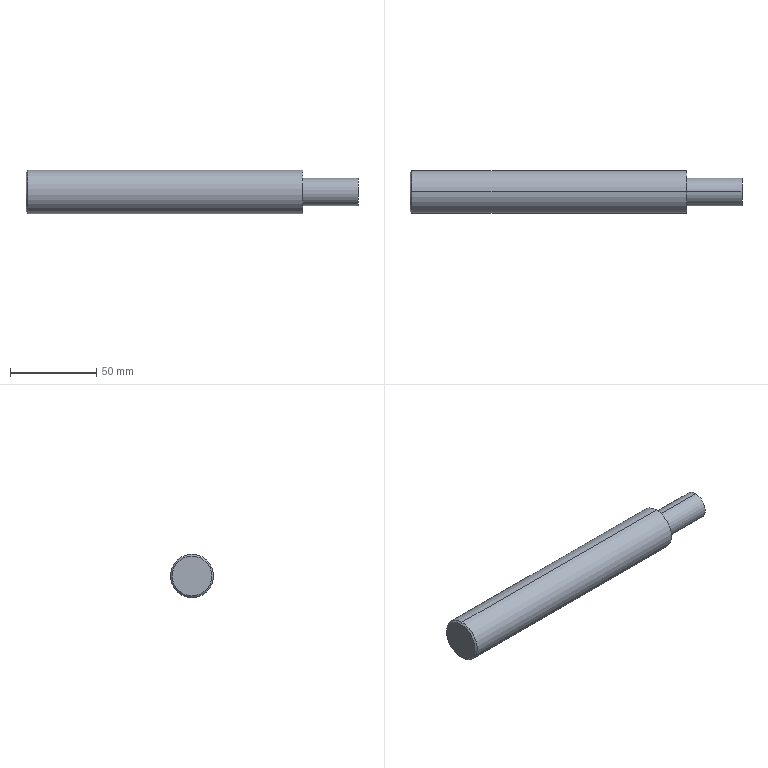Part | SolidWorks | features Chamfer 1, Revolution 1 | 1 solid | 9 faces | box 192 x 25 x 25 mm | volume 84936 mm3 | cylinder 4 | plane 3 | cone 2 | commonest cylinder face diameters 16 x2 25 x2
STEP:
#1=CARTESIAN_POINT('',(0.,0.,11.5));
#2=VERTEX_POINT('',#1);
#3=CARTESIAN_POINT('',(0.,0.,-11.5));
#4=VERTEX_POINT('',#3);
#5=CARTESIAN_POINT('',(0.,0.,0.));
#6=DIRECTION('',(-1.,0.,0.));
#7=DIRECTION('',(0.,0.,-1.));
#8=AXIS2_PLACEMENT_3D('',#5,#6,#7);
#9=CIRCLE('',#8,11.5);
#10=EDGE_CURVE('',#2,#4,#9,.T.);
#11=ORIENTED_EDGE('',*,*,#10,.F.);
#12=CARTESIAN_POINT('',(1.,0.,12.5));
#13=VERTEX_POINT('',#12);
#14=CARTESIAN_POINT('',(0.,0.,11.5));
#15=DIRECTION('',(0.7071,0.,0.7071));
#16=VECTOR('',#15,1000.);
#17=LINE('',#14,#16);
#18=EDGE_CURVE('',#2,#13,#17,.T.);
#19=ORIENTED_EDGE('',*,*,#18,.T.);
#20=CARTESIAN_POINT('',(1.,0.,-12.5));
#21=VERTEX_POINT('',#20);
#22=CARTESIAN_POINT('',(1.,0.,0.));
#23=DIRECTION('',(1.,0.,0.));
#24=DIRECTION('',(0.,0.,-1.));
#25=AXIS2_PLACEMENT_3D('',#22,#23,#24);
#26=CIRCLE('',#25,12.5);
#27=EDGE_CURVE('',#21,#13,#26,.T.);
#28=ORIENTED_EDGE('',*,*,#27,.F.);
#29=CARTESIAN_POINT('',(0.,0.,-11.5));
#30=DIRECTION('',(0.7071,0.,-0.7071));
#31=VECTOR('',#30,1000.);
#32=LINE('',#29,#31);
#33=EDGE_CURVE('',#4,#21,#32,.T.);
#34=ORIENTED_EDGE('',*,*,#33,.F.);
#35=EDGE_LOOP('',(#11,#19,#28,#34));
#36=FACE_OUTER_BOUND('',#35,.T.);
#37=CARTESIAN_POINT('',(0.,0.,0.));
#38=DIRECTION('',(1.,0.,0.));
#39=DIRECTION('',(0.,0.,-1.));
#40=AXIS2_PLACEMENT_3D('',#37,#38,#39);
#41=CONICAL_SURFACE('',#40,11.5,0.7854);
#42=ADVANCED_FACE('',(#36),#41,.T.);
#43=CARTESIAN_POINT('',(192.,0.,8.));
#44=VERTEX_POINT('',#43);
#45=CARTESIAN_POINT('',(192.,0.,-8.));
#46=VERTEX_POINT('',#45);
#47=CARTESIAN_POINT('',(192.,0.,0.));
#48=DIRECTION('',(-1.,0.,0.));
#49=DIRECTION('',(0.,0.,1.));
#50=AXIS2_PLACEMENT_3D('',#47,#48,#49);
#51=CIRCLE('',#50,8.);
#52=EDGE_CURVE('',#44,#46,#51,.T.);
#53=ORIENTED_EDGE('',*,*,#52,.T.);
#54=CARTESIAN_POINT('',(160.,0.,-8.));
#55=VERTEX_POINT('',#54);
#56=CARTESIAN_POINT('',(0.,0.,-8.));
#57=DIRECTION('',(-1.,0.,0.));
#58=VECTOR('',#57,1000.);
#59=LINE('',#56,#58);
#60=EDGE_CURVE('',#46,#55,#59,.T.);
#61=ORIENTED_EDGE('',*,*,#60,.T.);
#62=CARTESIAN_POINT('',(160.,0.,8.));
#63=VERTEX_POINT('',#62);
#64=CARTESIAN_POINT('',(160.,0.,0.));
#65=DIRECTION('',(-1.,0.,0.));
#66=DIRECTION('',(0.,0.,1.));
#67=AXIS2_PLACEMENT_3D('',#64,#65,#66);
#68=CIRCLE('',#67,8.);
#69=EDGE_CURVE('',#63,#55,#68,.T.);
#70=ORIENTED_EDGE('',*,*,#69,.F.);
#71=CARTESIAN_POINT('',(0.,0.,8.));
#72=DIRECTION('',(-1.,0.,0.));
#73=VECTOR('',#72,1000.);
#74=LINE('',#71,#73);
#75=EDGE_CURVE('',#44,#63,#74,.T.);
#76=ORIENTED_EDGE('',*,*,#75,.F.);
#77=EDGE_LOOP('',(#53,#61,#70,#76));
#78=FACE_OUTER_BOUND('',#77,.T.);
#79=CARTESIAN_POINT('',(0.,0.,0.));
#80=DIRECTION('',(-1.,0.,0.));
#81=DIRECTION('',(0.,0.,1.));
#82=AXIS2_PLACEMENT_3D('',#79,#80,#81);
#83=CYLINDRICAL_SURFACE('',#82,8.);
#84=ADVANCED_FACE('',(#78),#83,.T.);
#85=CARTESIAN_POINT('',(160.,0.,12.5));
#86=VERTEX_POINT('',#85);
#87=CARTESIAN_POINT('',(160.,0.,-12.5));
#88=VERTEX_POINT('',#87);
#89=CARTESIAN_POINT('',(160.,0.,0.));
#90=DIRECTION('',(-1.,0.,0.));
#91=DIRECTION('',(0.,0.,1.));
#92=AXIS2_PLACEMENT_3D('',#89,#90,#91);
#93=CIRCLE('',#92,12.5);
#94=EDGE_CURVE('',#86,#88,#93,.T.);
#95=ORIENTED_EDGE('',*,*,#94,.T.);
#96=CARTESIAN_POINT('',(0.,0.,-12.5));
#97=DIRECTION('',(-1.,0.,0.));
#98=VECTOR('',#97,1000.);
#99=LINE('',#96,#98);
#100=EDGE_CURVE('',#88,#21,#99,.T.);
#101=ORIENTED_EDGE('',*,*,#100,.T.);
#102=ORIENTED_EDGE('',*,*,#27,.T.);
#103=CARTESIAN_POINT('',(0.,0.,12.5));
#104=DIRECTION('',(-1.,0.,0.));
#105=VECTOR('',#104,1000.);
#106=LINE('',#103,#105);
#107=EDGE_CURVE('',#86,#13,#106,.T.);
#108=ORIENTED_EDGE('',*,*,#107,.F.);
#109=EDGE_LOOP('',(#95,#101,#102,#108));
#110=FACE_OUTER_BOUND('',#109,.T.);
#111=CARTESIAN_POINT('',(0.,0.,0.));
#112=DIRECTION('',(-1.,0.,0.));
#113=DIRECTION('',(0.,0.,1.));
#114=AXIS2_PLACEMENT_3D('',#111,#112,#113);
#115=CYLINDRICAL_SURFACE('',#114,12.5);
#116=ADVANCED_FACE('',(#110),#115,.T.);
#117=CARTESIAN_POINT('',(0.,0.,0.));
#118=DIRECTION('',(-1.,0.,0.));
#119=DIRECTION('',(0.,0.,-1.));
#120=AXIS2_PLACEMENT_3D('',#117,#118,#119);
#121=CIRCLE('',#120,11.5);
#122=EDGE_CURVE('',#4,#2,#121,.T.);
#123=ORIENTED_EDGE('',*,*,#122,.T.);
#124=ORIENTED_EDGE('',*,*,#10,.T.);
#125=EDGE_LOOP('',(#123,#124));
#126=FACE_OUTER_BOUND('',#125,.T.);
#127=CARTESIAN_POINT('',(0.,0.,0.));
#128=DIRECTION('',(1.,0.,0.));
#129=DIRECTION('',(0.,0.,-1.));
#130=AXIS2_PLACEMENT_3D('',#127,#128,#129);
#131=PLANE('',#130);
#132=ADVANCED_FACE('',(#126),#131,.F.);
#133=ORIENTED_EDGE('',*,*,#100,.F.);
#134=CARTESIAN_POINT('',(160.,0.,0.));
#135=DIRECTION('',(-1.,0.,0.));
#136=DIRECTION('',(0.,0.,1.));
#137=AXIS2_PLACEMENT_3D('',#134,#135,#136);
#138=CIRCLE('',#137,12.5);
#139=EDGE_CURVE('',#88,#86,#138,.T.);
#140=ORIENTED_EDGE('',*,*,#139,.T.);
#141=ORIENTED_EDGE('',*,*,#107,.T.);
#142=CARTESIAN_POINT('',(1.,0.,0.));
#143=DIRECTION('',(1.,0.,0.));
#144=DIRECTION('',(0.,0.,-1.));
#145=AXIS2_PLACEMENT_3D('',#142,#143,#144);
#146=CIRCLE('',#145,12.5);
#147=EDGE_CURVE('',#13,#21,#146,.T.);
#148=ORIENTED_EDGE('',*,*,#147,.T.);
#149=EDGE_LOOP('',(#133,#140,#141,#148));
#150=FACE_OUTER_BOUND('',#149,.T.);
#151=CARTESIAN_POINT('',(0.,0.,0.));
#152=DIRECTION('',(-1.,0.,0.));
#153=DIRECTION('',(0.,0.,1.));
#154=AXIS2_PLACEMENT_3D('',#151,#152,#153);
#155=CYLINDRICAL_SURFACE('',#154,12.5);
#156=ADVANCED_FACE('',(#150),#155,.T.);
#157=ORIENTED_EDGE('',*,*,#94,.F.);
#158=ORIENTED_EDGE('',*,*,#139,.F.);
#159=EDGE_LOOP('',(#157,#158));
#160=FACE_OUTER_BOUND('',#159,.T.);
#161=ORIENTED_EDGE('',*,*,#69,.T.);
#162=CARTESIAN_POINT('',(160.,0.,0.));
#163=DIRECTION('',(-1.,0.,0.));
#164=DIRECTION('',(0.,0.,1.));
#165=AXIS2_PLACEMENT_3D('',#162,#163,#164);
#166=CIRCLE('',#165,8.);
#167=EDGE_CURVE('',#55,#63,#166,.T.);
#168=ORIENTED_EDGE('',*,*,#167,.T.);
#169=EDGE_LOOP('',(#161,#168));
#170=FACE_BOUND('',#169,.T.);
#171=CARTESIAN_POINT('',(160.,12.5,0.));
#172=DIRECTION('',(-1.,0.,0.));
#173=DIRECTION('',(0.,0.,1.));
#174=AXIS2_PLACEMENT_3D('',#171,#172,#173);
#175=PLANE('',#174);
#176=ADVANCED_FACE('',(#160,#170),#175,.F.);
#177=ORIENTED_EDGE('',*,*,#60,.F.);
#178=CARTESIAN_POINT('',(192.,0.,0.));
#179=DIRECTION('',(-1.,0.,0.));
#180=DIRECTION('',(0.,0.,1.));
#181=AXIS2_PLACEMENT_3D('',#178,#179,#180);
#182=CIRCLE('',#181,8.);
#183=EDGE_CURVE('',#46,#44,#182,.T.);
#184=ORIENTED_EDGE('',*,*,#183,.T.);
#185=ORIENTED_EDGE('',*,*,#75,.T.);
#186=ORIENTED_EDGE('',*,*,#167,.F.);
#187=EDGE_LOOP('',(#177,#184,#185,#186));
#188=FACE_OUTER_BOUND('',#187,.T.);
#189=CARTESIAN_POINT('',(0.,0.,0.));
#190=DIRECTION('',(-1.,0.,0.));
#191=DIRECTION('',(0.,0.,1.));
#192=AXIS2_PLACEMENT_3D('',#189,#190,#191);
#193=CYLINDRICAL_SURFACE('',#192,8.);
#194=ADVANCED_FACE('',(#188),#193,.T.);
#195=ORIENTED_EDGE('',*,*,#52,.F.);
#196=ORIENTED_EDGE('',*,*,#183,.F.);
#197=EDGE_LOOP('',(#195,#196));
#198=FACE_OUTER_BOUND('',#197,.T.);
#199=CARTESIAN_POINT('',(192.,8.,0.));
#200=DIRECTION('',(-1.,0.,0.));
#201=DIRECTION('',(0.,0.,1.));
#202=AXIS2_PLACEMENT_3D('',#199,#200,#201);
#203=PLANE('',#202);
#204=ADVANCED_FACE('',(#198),#203,.F.);
#205=ORIENTED_EDGE('',*,*,#18,.F.);
#206=ORIENTED_EDGE('',*,*,#122,.F.);
#207=ORIENTED_EDGE('',*,*,#33,.T.);
#208=ORIENTED_EDGE('',*,*,#147,.F.);
#209=EDGE_LOOP('',(#205,#206,#207,#208));
#210=FACE_OUTER_BOUND('',#209,.T.);
#211=CARTESIAN_POINT('',(0.,0.,0.));
#212=DIRECTION('',(1.,0.,0.));
#213=DIRECTION('',(0.,0.,-1.));
#214=AXIS2_PLACEMENT_3D('',#211,#212,#213);
#215=CONICAL_SURFACE('',#214,11.5,0.7854);
#216=ADVANCED_FACE('',(#210),#215,.T.);
#217=CLOSED_SHELL('',(#42,#84,#116,#132,#156,#176,#194,#204,#216));
#218=MANIFOLD_SOLID_BREP('',#217);
#219=CARTESIAN_POINT('',(0.,0.,0.));
#220=DIRECTION('',(0.,0.,1.));
#221=DIRECTION('',(1.,0.,0.));
#222=AXIS2_PLACEMENT_3D('',#219,#220,#221);
#223=(LENGTH_UNIT()NAMED_UNIT(*)SI_UNIT(.MILLI.,.METRE.));
#224=UNCERTAINTY_MEASURE_WITH_UNIT(LENGTH_MEASURE(0.00001),#223,'','');
#225=(NAMED_UNIT(*)PLANE_ANGLE_UNIT()SI_UNIT($,.RADIAN.));
#226=(NAMED_UNIT(*)SI_UNIT($,.STERADIAN.)SOLID_ANGLE_UNIT());
#227=(GEOMETRIC_REPRESENTATION_CONTEXT(3)GLOBAL_UNCERTAINTY_ASSIGNED_CONTEXT((#224))GLOBAL_UNIT_ASSIGNED_CONTEXT((#223,#225,#226))REPRESENTATION_CONTEXT('',''));
#228=ADVANCED_BREP_SHAPE_REPRESENTATION('',(#218,#222),#227);